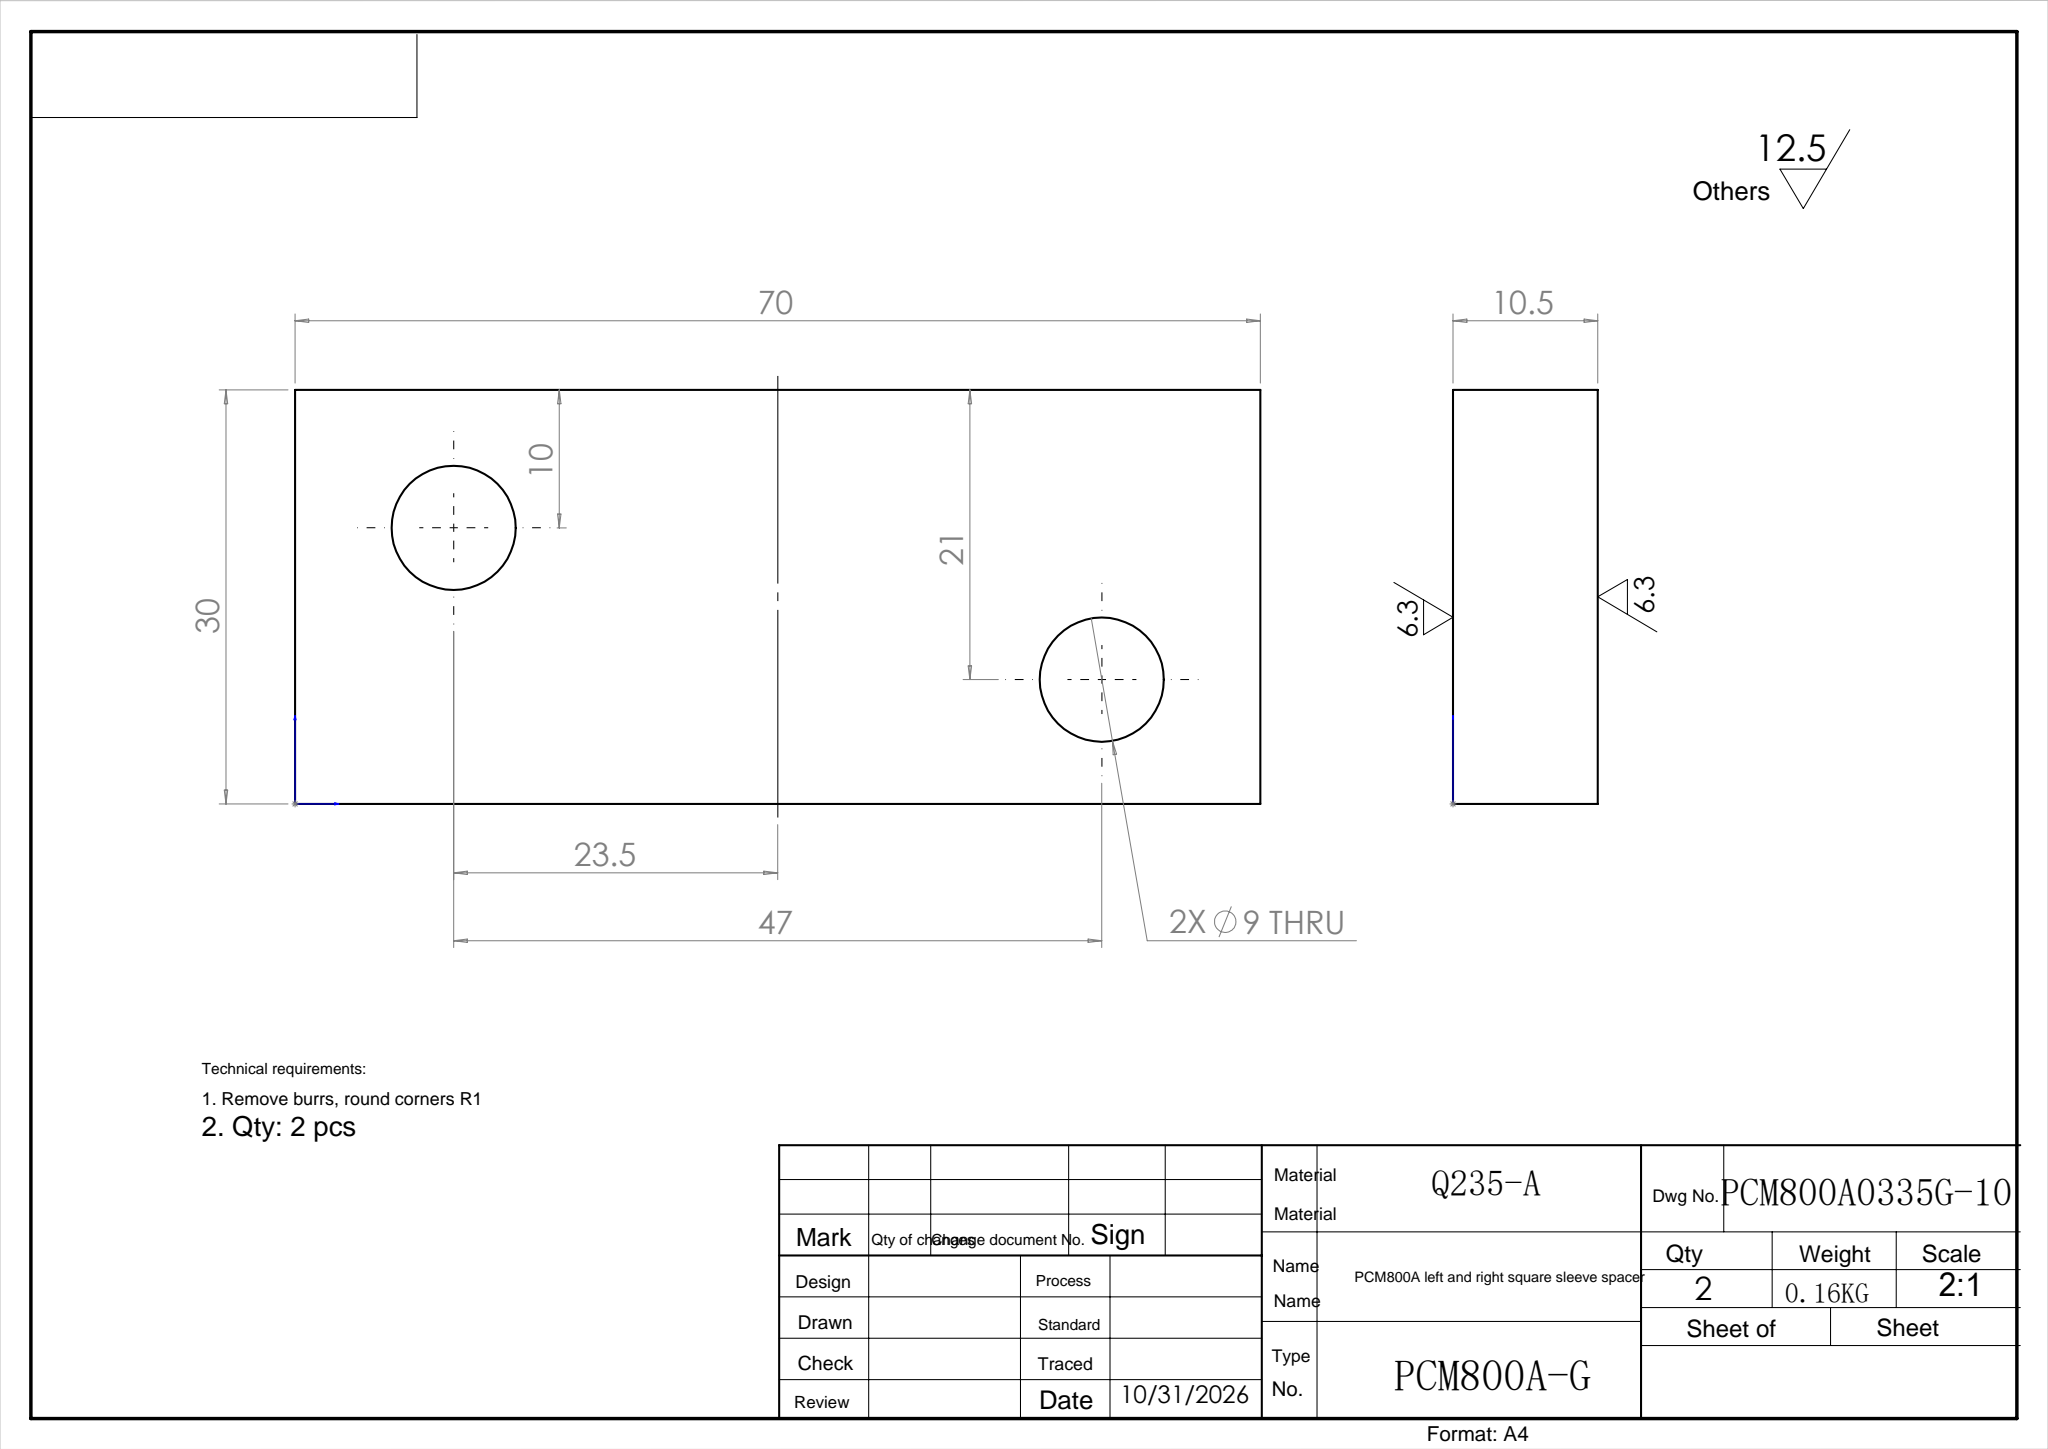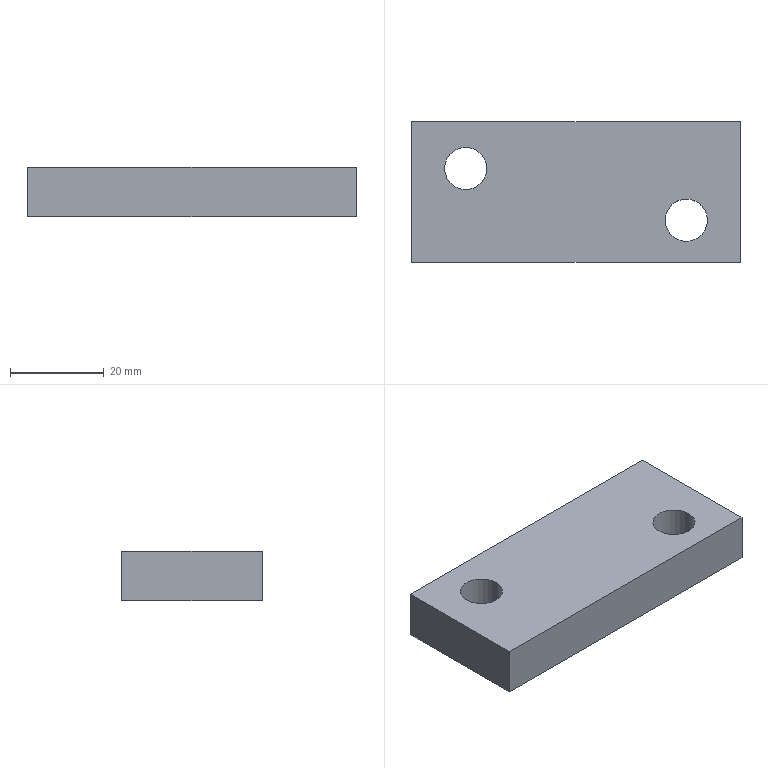Part | SolidWorks | features Extrusion 1 | 1 solid | 10 faces | box 70 x 30 x 10.5 mm | volume 20714 mm3 | plane 6 | cylinder 4 | commonest cylinder face diameters 9 x4
STEP:
#1=CARTESIAN_POINT('',(54.,9.,10.5));
#2=VERTEX_POINT('',#1);
#3=CARTESIAN_POINT('',(63.,9.,10.5));
#4=VERTEX_POINT('',#3);
#5=CARTESIAN_POINT('',(58.5,9.,10.5));
#6=DIRECTION('',(0.,0.,1.));
#7=DIRECTION('',(1.,0.,0.));
#8=AXIS2_PLACEMENT_3D('',#5,#6,#7);
#9=CIRCLE('',#8,4.5);
#10=EDGE_CURVE('',#2,#4,#9,.T.);
#11=ORIENTED_EDGE('',*,*,#10,.T.);
#12=CARTESIAN_POINT('',(63.,9.,0.));
#13=VERTEX_POINT('',#12);
#14=CARTESIAN_POINT('',(63.,9.,10.5));
#15=DIRECTION('',(0.,0.,-1.));
#16=VECTOR('',#15,1000.);
#17=LINE('',#14,#16);
#18=EDGE_CURVE('',#4,#13,#17,.T.);
#19=ORIENTED_EDGE('',*,*,#18,.T.);
#20=CARTESIAN_POINT('',(54.,9.,0.));
#21=VERTEX_POINT('',#20);
#22=CARTESIAN_POINT('',(58.5,9.,0.));
#23=DIRECTION('',(0.,0.,1.));
#24=DIRECTION('',(1.,0.,0.));
#25=AXIS2_PLACEMENT_3D('',#22,#23,#24);
#26=CIRCLE('',#25,4.5);
#27=EDGE_CURVE('',#21,#13,#26,.T.);
#28=ORIENTED_EDGE('',*,*,#27,.F.);
#29=CARTESIAN_POINT('',(54.,9.,10.5));
#30=DIRECTION('',(0.,0.,-1.));
#31=VECTOR('',#30,1000.);
#32=LINE('',#29,#31);
#33=EDGE_CURVE('',#2,#21,#32,.T.);
#34=ORIENTED_EDGE('',*,*,#33,.F.);
#35=EDGE_LOOP('',(#11,#19,#28,#34));
#36=FACE_OUTER_BOUND('',#35,.T.);
#37=CARTESIAN_POINT('',(58.5,9.,10.5));
#38=DIRECTION('',(0.,0.,-1.));
#39=DIRECTION('',(-1.,0.,0.));
#40=AXIS2_PLACEMENT_3D('',#37,#38,#39);
#41=CYLINDRICAL_SURFACE('',#40,4.5);
#42=ADVANCED_FACE('',(#36),#41,.F.);
#43=CARTESIAN_POINT('',(7.,20.,10.5));
#44=VERTEX_POINT('',#43);
#45=CARTESIAN_POINT('',(16.,20.,10.5));
#46=VERTEX_POINT('',#45);
#47=CARTESIAN_POINT('',(11.5,20.,10.5));
#48=DIRECTION('',(0.,0.,1.));
#49=DIRECTION('',(1.,0.,0.));
#50=AXIS2_PLACEMENT_3D('',#47,#48,#49);
#51=CIRCLE('',#50,4.5);
#52=EDGE_CURVE('',#44,#46,#51,.T.);
#53=ORIENTED_EDGE('',*,*,#52,.T.);
#54=CARTESIAN_POINT('',(16.,20.,0.));
#55=VERTEX_POINT('',#54);
#56=CARTESIAN_POINT('',(16.,20.,10.5));
#57=DIRECTION('',(0.,0.,-1.));
#58=VECTOR('',#57,1000.);
#59=LINE('',#56,#58);
#60=EDGE_CURVE('',#46,#55,#59,.T.);
#61=ORIENTED_EDGE('',*,*,#60,.T.);
#62=CARTESIAN_POINT('',(7.,20.,0.));
#63=VERTEX_POINT('',#62);
#64=CARTESIAN_POINT('',(11.5,20.,0.));
#65=DIRECTION('',(0.,0.,1.));
#66=DIRECTION('',(1.,0.,0.));
#67=AXIS2_PLACEMENT_3D('',#64,#65,#66);
#68=CIRCLE('',#67,4.5);
#69=EDGE_CURVE('',#63,#55,#68,.T.);
#70=ORIENTED_EDGE('',*,*,#69,.F.);
#71=CARTESIAN_POINT('',(7.,20.,10.5));
#72=DIRECTION('',(0.,0.,-1.));
#73=VECTOR('',#72,1000.);
#74=LINE('',#71,#73);
#75=EDGE_CURVE('',#44,#63,#74,.T.);
#76=ORIENTED_EDGE('',*,*,#75,.F.);
#77=EDGE_LOOP('',(#53,#61,#70,#76));
#78=FACE_OUTER_BOUND('',#77,.T.);
#79=CARTESIAN_POINT('',(11.5,20.,10.5));
#80=DIRECTION('',(0.,0.,-1.));
#81=DIRECTION('',(-1.,0.,0.));
#82=AXIS2_PLACEMENT_3D('',#79,#80,#81);
#83=CYLINDRICAL_SURFACE('',#82,4.5);
#84=ADVANCED_FACE('',(#78),#83,.F.);
#85=ORIENTED_EDGE('',*,*,#52,.F.);
#86=CARTESIAN_POINT('',(11.5,20.,10.5));
#87=DIRECTION('',(0.,0.,1.));
#88=DIRECTION('',(1.,0.,0.));
#89=AXIS2_PLACEMENT_3D('',#86,#87,#88);
#90=CIRCLE('',#89,4.5);
#91=EDGE_CURVE('',#46,#44,#90,.T.);
#92=ORIENTED_EDGE('',*,*,#91,.F.);
#93=EDGE_LOOP('',(#85,#92));
#94=FACE_BOUND('',#93,.T.);
#95=CARTESIAN_POINT('',(0.,30.,10.5));
#96=VERTEX_POINT('',#95);
#97=CARTESIAN_POINT('',(0.,0.,10.5));
#98=VERTEX_POINT('',#97);
#99=CARTESIAN_POINT('',(0.,0.,10.5));
#100=DIRECTION('',(0.,-1.,0.));
#101=VECTOR('',#100,1000.);
#102=LINE('',#99,#101);
#103=EDGE_CURVE('',#96,#98,#102,.T.);
#104=ORIENTED_EDGE('',*,*,#103,.T.);
#105=CARTESIAN_POINT('',(70.,0.,10.5));
#106=VERTEX_POINT('',#105);
#107=CARTESIAN_POINT('',(0.,0.,10.5));
#108=DIRECTION('',(1.,0.,0.));
#109=VECTOR('',#108,1000.);
#110=LINE('',#107,#109);
#111=EDGE_CURVE('',#98,#106,#110,.T.);
#112=ORIENTED_EDGE('',*,*,#111,.T.);
#113=CARTESIAN_POINT('',(70.,30.,10.5));
#114=VERTEX_POINT('',#113);
#115=CARTESIAN_POINT('',(70.,0.,10.5));
#116=DIRECTION('',(0.,1.,0.));
#117=VECTOR('',#116,1000.);
#118=LINE('',#115,#117);
#119=EDGE_CURVE('',#106,#114,#118,.T.);
#120=ORIENTED_EDGE('',*,*,#119,.T.);
#121=CARTESIAN_POINT('',(0.,30.,10.5));
#122=DIRECTION('',(-1.,0.,0.));
#123=VECTOR('',#122,1000.);
#124=LINE('',#121,#123);
#125=EDGE_CURVE('',#114,#96,#124,.T.);
#126=ORIENTED_EDGE('',*,*,#125,.T.);
#127=EDGE_LOOP('',(#104,#112,#120,#126));
#128=FACE_OUTER_BOUND('',#127,.T.);
#129=ORIENTED_EDGE('',*,*,#10,.F.);
#130=CARTESIAN_POINT('',(58.5,9.,10.5));
#131=DIRECTION('',(0.,0.,1.));
#132=DIRECTION('',(1.,0.,0.));
#133=AXIS2_PLACEMENT_3D('',#130,#131,#132);
#134=CIRCLE('',#133,4.5);
#135=EDGE_CURVE('',#4,#2,#134,.T.);
#136=ORIENTED_EDGE('',*,*,#135,.F.);
#137=EDGE_LOOP('',(#129,#136));
#138=FACE_BOUND('',#137,.T.);
#139=CARTESIAN_POINT('',(0.,30.,10.5));
#140=DIRECTION('',(0.,0.,-1.));
#141=DIRECTION('',(-1.,0.,0.));
#142=AXIS2_PLACEMENT_3D('',#139,#140,#141);
#143=PLANE('',#142);
#144=ADVANCED_FACE('',(#94,#128,#138),#143,.F.);
#145=ORIENTED_EDGE('',*,*,#69,.T.);
#146=CARTESIAN_POINT('',(11.5,20.,0.));
#147=DIRECTION('',(0.,0.,1.));
#148=DIRECTION('',(1.,0.,0.));
#149=AXIS2_PLACEMENT_3D('',#146,#147,#148);
#150=CIRCLE('',#149,4.5);
#151=EDGE_CURVE('',#55,#63,#150,.T.);
#152=ORIENTED_EDGE('',*,*,#151,.T.);
#153=EDGE_LOOP('',(#145,#152));
#154=FACE_BOUND('',#153,.T.);
#155=CARTESIAN_POINT('',(0.,30.,0.));
#156=VERTEX_POINT('',#155);
#157=CARTESIAN_POINT('',(0.,0.,0.));
#158=VERTEX_POINT('',#157);
#159=CARTESIAN_POINT('',(0.,0.,0.));
#160=DIRECTION('',(0.,-1.,0.));
#161=VECTOR('',#160,1000.);
#162=LINE('',#159,#161);
#163=EDGE_CURVE('',#156,#158,#162,.T.);
#164=ORIENTED_EDGE('',*,*,#163,.F.);
#165=CARTESIAN_POINT('',(70.,30.,0.));
#166=VERTEX_POINT('',#165);
#167=CARTESIAN_POINT('',(0.,30.,0.));
#168=DIRECTION('',(-1.,0.,0.));
#169=VECTOR('',#168,1000.);
#170=LINE('',#167,#169);
#171=EDGE_CURVE('',#166,#156,#170,.T.);
#172=ORIENTED_EDGE('',*,*,#171,.F.);
#173=CARTESIAN_POINT('',(70.,0.,0.));
#174=VERTEX_POINT('',#173);
#175=CARTESIAN_POINT('',(70.,0.,0.));
#176=DIRECTION('',(0.,1.,0.));
#177=VECTOR('',#176,1000.);
#178=LINE('',#175,#177);
#179=EDGE_CURVE('',#174,#166,#178,.T.);
#180=ORIENTED_EDGE('',*,*,#179,.F.);
#181=CARTESIAN_POINT('',(0.,0.,0.));
#182=DIRECTION('',(1.,0.,0.));
#183=VECTOR('',#182,1000.);
#184=LINE('',#181,#183);
#185=EDGE_CURVE('',#158,#174,#184,.T.);
#186=ORIENTED_EDGE('',*,*,#185,.F.);
#187=EDGE_LOOP('',(#164,#172,#180,#186));
#188=FACE_OUTER_BOUND('',#187,.T.);
#189=ORIENTED_EDGE('',*,*,#27,.T.);
#190=CARTESIAN_POINT('',(58.5,9.,0.));
#191=DIRECTION('',(0.,0.,1.));
#192=DIRECTION('',(1.,0.,0.));
#193=AXIS2_PLACEMENT_3D('',#190,#191,#192);
#194=CIRCLE('',#193,4.5);
#195=EDGE_CURVE('',#13,#21,#194,.T.);
#196=ORIENTED_EDGE('',*,*,#195,.T.);
#197=EDGE_LOOP('',(#189,#196));
#198=FACE_BOUND('',#197,.T.);
#199=CARTESIAN_POINT('',(0.,30.,0.));
#200=DIRECTION('',(0.,0.,-1.));
#201=DIRECTION('',(-1.,0.,0.));
#202=AXIS2_PLACEMENT_3D('',#199,#200,#201);
#203=PLANE('',#202);
#204=ADVANCED_FACE('',(#154,#188,#198),#203,.T.);
#205=ORIENTED_EDGE('',*,*,#163,.T.);
#206=CARTESIAN_POINT('',(0.,0.,10.5));
#207=DIRECTION('',(0.,0.,-1.));
#208=VECTOR('',#207,1000.);
#209=LINE('',#206,#208);
#210=EDGE_CURVE('',#98,#158,#209,.T.);
#211=ORIENTED_EDGE('',*,*,#210,.F.);
#212=ORIENTED_EDGE('',*,*,#103,.F.);
#213=CARTESIAN_POINT('',(0.,30.,10.5));
#214=DIRECTION('',(0.,0.,-1.));
#215=VECTOR('',#214,1000.);
#216=LINE('',#213,#215);
#217=EDGE_CURVE('',#96,#156,#216,.T.);
#218=ORIENTED_EDGE('',*,*,#217,.T.);
#219=EDGE_LOOP('',(#205,#211,#212,#218));
#220=FACE_OUTER_BOUND('',#219,.T.);
#221=CARTESIAN_POINT('',(0.,0.,10.5));
#222=DIRECTION('',(1.,0.,0.));
#223=DIRECTION('',(0.,0.,-1.));
#224=AXIS2_PLACEMENT_3D('',#221,#222,#223);
#225=PLANE('',#224);
#226=ADVANCED_FACE('',(#220),#225,.F.);
#227=ORIENTED_EDGE('',*,*,#185,.T.);
#228=CARTESIAN_POINT('',(70.,0.,10.5));
#229=DIRECTION('',(0.,0.,-1.));
#230=VECTOR('',#229,1000.);
#231=LINE('',#228,#230);
#232=EDGE_CURVE('',#106,#174,#231,.T.);
#233=ORIENTED_EDGE('',*,*,#232,.F.);
#234=ORIENTED_EDGE('',*,*,#111,.F.);
#235=ORIENTED_EDGE('',*,*,#210,.T.);
#236=EDGE_LOOP('',(#227,#233,#234,#235));
#237=FACE_OUTER_BOUND('',#236,.T.);
#238=CARTESIAN_POINT('',(0.,0.,10.5));
#239=DIRECTION('',(0.,1.,0.));
#240=DIRECTION('',(0.,0.,1.));
#241=AXIS2_PLACEMENT_3D('',#238,#239,#240);
#242=PLANE('',#241);
#243=ADVANCED_FACE('',(#237),#242,.F.);
#244=ORIENTED_EDGE('',*,*,#179,.T.);
#245=CARTESIAN_POINT('',(70.,30.,10.5));
#246=DIRECTION('',(0.,0.,-1.));
#247=VECTOR('',#246,1000.);
#248=LINE('',#245,#247);
#249=EDGE_CURVE('',#114,#166,#248,.T.);
#250=ORIENTED_EDGE('',*,*,#249,.F.);
#251=ORIENTED_EDGE('',*,*,#119,.F.);
#252=ORIENTED_EDGE('',*,*,#232,.T.);
#253=EDGE_LOOP('',(#244,#250,#251,#252));
#254=FACE_OUTER_BOUND('',#253,.T.);
#255=CARTESIAN_POINT('',(70.,0.,10.5));
#256=DIRECTION('',(-1.,0.,0.));
#257=DIRECTION('',(0.,0.,1.));
#258=AXIS2_PLACEMENT_3D('',#255,#256,#257);
#259=PLANE('',#258);
#260=ADVANCED_FACE('',(#254),#259,.F.);
#261=ORIENTED_EDGE('',*,*,#171,.T.);
#262=ORIENTED_EDGE('',*,*,#217,.F.);
#263=ORIENTED_EDGE('',*,*,#125,.F.);
#264=ORIENTED_EDGE('',*,*,#249,.T.);
#265=EDGE_LOOP('',(#261,#262,#263,#264));
#266=FACE_OUTER_BOUND('',#265,.T.);
#267=CARTESIAN_POINT('',(0.,30.,10.5));
#268=DIRECTION('',(0.,-1.,0.));
#269=DIRECTION('',(0.,0.,-1.));
#270=AXIS2_PLACEMENT_3D('',#267,#268,#269);
#271=PLANE('',#270);
#272=ADVANCED_FACE('',(#266),#271,.F.);
#273=ORIENTED_EDGE('',*,*,#60,.F.);
#274=ORIENTED_EDGE('',*,*,#91,.T.);
#275=ORIENTED_EDGE('',*,*,#75,.T.);
#276=ORIENTED_EDGE('',*,*,#151,.F.);
#277=EDGE_LOOP('',(#273,#274,#275,#276));
#278=FACE_OUTER_BOUND('',#277,.T.);
#279=CARTESIAN_POINT('',(11.5,20.,10.5));
#280=DIRECTION('',(0.,0.,-1.));
#281=DIRECTION('',(-1.,0.,0.));
#282=AXIS2_PLACEMENT_3D('',#279,#280,#281);
#283=CYLINDRICAL_SURFACE('',#282,4.5);
#284=ADVANCED_FACE('',(#278),#283,.F.);
#285=ORIENTED_EDGE('',*,*,#18,.F.);
#286=ORIENTED_EDGE('',*,*,#135,.T.);
#287=ORIENTED_EDGE('',*,*,#33,.T.);
#288=ORIENTED_EDGE('',*,*,#195,.F.);
#289=EDGE_LOOP('',(#285,#286,#287,#288));
#290=FACE_OUTER_BOUND('',#289,.T.);
#291=CARTESIAN_POINT('',(58.5,9.,10.5));
#292=DIRECTION('',(0.,0.,-1.));
#293=DIRECTION('',(-1.,0.,0.));
#294=AXIS2_PLACEMENT_3D('',#291,#292,#293);
#295=CYLINDRICAL_SURFACE('',#294,4.5);
#296=ADVANCED_FACE('',(#290),#295,.F.);
#297=CLOSED_SHELL('',(#42,#84,#144,#204,#226,#243,#260,#272,#284,#296));
#298=MANIFOLD_SOLID_BREP('',#297);
#299=CARTESIAN_POINT('',(0.,0.,0.));
#300=DIRECTION('',(0.,0.,1.));
#301=DIRECTION('',(1.,0.,0.));
#302=AXIS2_PLACEMENT_3D('',#299,#300,#301);
#303=(LENGTH_UNIT()NAMED_UNIT(*)SI_UNIT(.MILLI.,.METRE.));
#304=UNCERTAINTY_MEASURE_WITH_UNIT(LENGTH_MEASURE(0.00001),#303,'','');
#305=(NAMED_UNIT(*)PLANE_ANGLE_UNIT()SI_UNIT($,.RADIAN.));
#306=(NAMED_UNIT(*)SI_UNIT($,.STERADIAN.)SOLID_ANGLE_UNIT());
#307=(GEOMETRIC_REPRESENTATION_CONTEXT(3)GLOBAL_UNCERTAINTY_ASSIGNED_CONTEXT((#304))GLOBAL_UNIT_ASSIGNED_CONTEXT((#303,#305,#306))REPRESENTATION_CONTEXT('',''));
#308=ADVANCED_BREP_SHAPE_REPRESENTATION('',(#298,#302),#307);